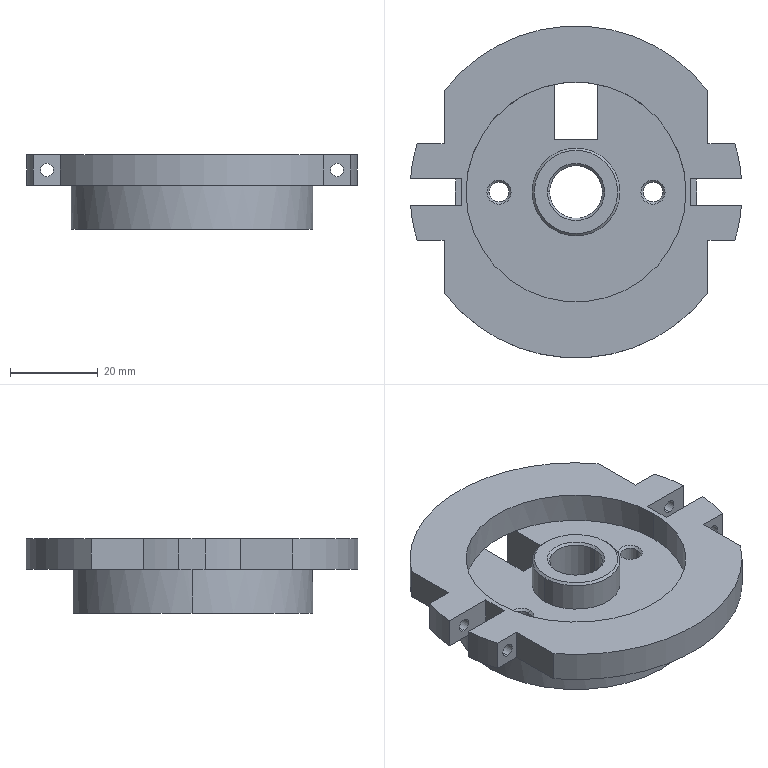Part | STEP file | PN_0094 limit stopper | 1 solid | 71 faces | box 75.261 x 75.5 x 17 mm | volume 37225 mm3 | cylinder 31 | plane 26 | cone 14 | commonest cylinder face diameters 3 x8 75.5 x6 4.5 x4 55 x3 4 x2 4.2 x2